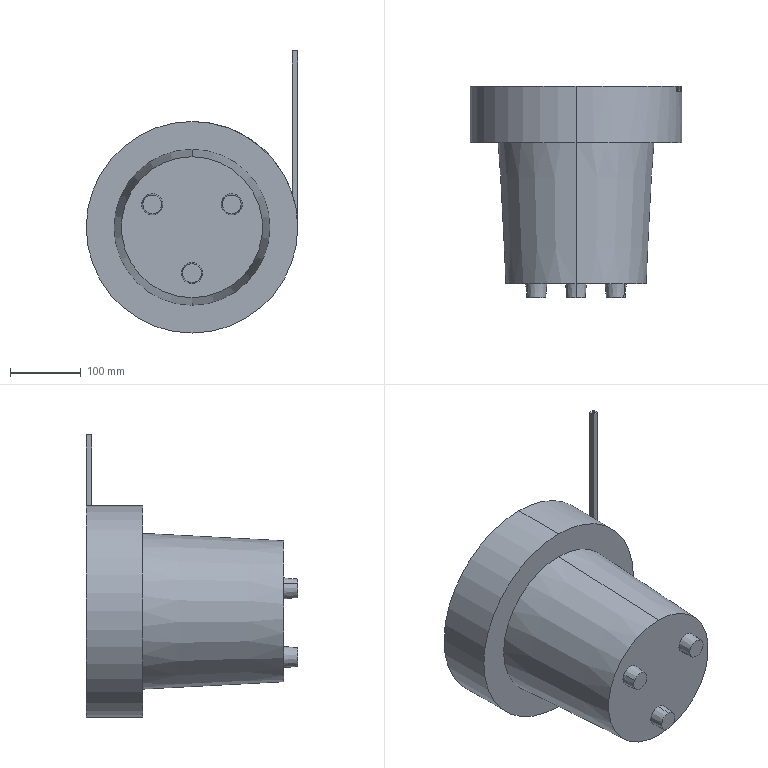Part | NX | features BREP 1 | 1 solid | 40 faces | box 300 x 300 x 400 mm | volume 553756 mm3 | plane 20 | cone 16 | cylinder 4 | commonest cylinder face diameters 296 x2 300 x2
STEP:
#1=CARTESIAN_POINT('',(66.18,-18.,38.209));
#2=VERTEX_POINT('',#1);
#3=CARTESIAN_POINT('',(46.404,-18.,26.791));
#4=VERTEX_POINT('',#3);
#5=CARTESIAN_POINT('',(56.292,-18.,32.5));
#6=DIRECTION('',(0.,-1.,0.));
#7=DIRECTION('',(0.,0.,-1.));
#8=AXIS2_PLACEMENT_3D('',#5,#6,#7);
#9=CIRCLE('',#8,11.418);
#10=EDGE_CURVE('',#2,#4,#9,.T.);
#11=ORIENTED_EDGE('',*,*,#10,.T.);
#12=CARTESIAN_POINT('',(44.888,2.,25.916));
#13=VERTEX_POINT('',#12);
#14=CARTESIAN_POINT('',(45.027,0.1743,25.996));
#15=DIRECTION('',(-0.07548,0.9962,-0.04358));
#16=VECTOR('',#15,1000.);
#17=LINE('',#14,#16);
#18=EDGE_CURVE('',#13,#4,#17,.F.);
#19=ORIENTED_EDGE('',*,*,#18,.F.);
#20=CARTESIAN_POINT('',(67.695,2.,39.084));
#21=VERTEX_POINT('',#20);
#22=CARTESIAN_POINT('',(56.292,2.,32.5));
#23=DIRECTION('',(0.,-1.,0.));
#24=DIRECTION('',(0.,0.,1.));
#25=AXIS2_PLACEMENT_3D('',#22,#23,#24);
#26=CIRCLE('',#25,13.167);
#27=EDGE_CURVE('',#21,#13,#26,.T.);
#28=ORIENTED_EDGE('',*,*,#27,.F.);
#29=CARTESIAN_POINT('',(67.557,0.1743,39.004));
#30=DIRECTION('',(0.07548,0.9962,0.04358));
#31=VECTOR('',#30,1000.);
#32=LINE('',#29,#31);
#33=EDGE_CURVE('',#21,#2,#32,.F.);
#34=ORIENTED_EDGE('',*,*,#33,.T.);
#35=EDGE_LOOP('',(#11,#19,#28,#34));
#36=FACE_BOUND('',#35,.T.);
#37=CARTESIAN_POINT('',(56.292,0.1743,32.5));
#38=DIRECTION('',(0.,1.,0.));
#39=DIRECTION('',(0.866,0.,0.5));
#40=AXIS2_PLACEMENT_3D('',#37,#38,#39);
#41=CONICAL_SURFACE('',#40,13.008,0.08727);
#42=ADVANCED_FACE('',(#36),#41,.F.);
#43=CARTESIAN_POINT('',(-66.18,-18.,38.209));
#44=VERTEX_POINT('',#43);
#45=CARTESIAN_POINT('',(-46.404,-18.,26.791));
#46=VERTEX_POINT('',#45);
#47=CARTESIAN_POINT('',(-56.292,-18.,32.5));
#48=DIRECTION('',(0.,-1.,0.));
#49=DIRECTION('',(0.,0.,-1.));
#50=AXIS2_PLACEMENT_3D('',#47,#48,#49);
#51=CIRCLE('',#50,11.418);
#52=EDGE_CURVE('',#44,#46,#51,.T.);
#53=ORIENTED_EDGE('',*,*,#52,.T.);
#54=CARTESIAN_POINT('',(-44.888,2.,25.916));
#55=VERTEX_POINT('',#54);
#56=CARTESIAN_POINT('',(-45.027,0.1743,25.996));
#57=DIRECTION('',(0.07548,0.9962,-0.04358));
#58=VECTOR('',#57,1000.);
#59=LINE('',#56,#58);
#60=EDGE_CURVE('',#46,#55,#59,.T.);
#61=ORIENTED_EDGE('',*,*,#60,.T.);
#62=CARTESIAN_POINT('',(-67.695,2.,39.084));
#63=VERTEX_POINT('',#62);
#64=CARTESIAN_POINT('',(-56.292,2.,32.5));
#65=DIRECTION('',(0.,-1.,0.));
#66=DIRECTION('',(0.,0.,1.));
#67=AXIS2_PLACEMENT_3D('',#64,#65,#66);
#68=CIRCLE('',#67,13.167);
#69=EDGE_CURVE('',#63,#55,#68,.T.);
#70=ORIENTED_EDGE('',*,*,#69,.F.);
#71=CARTESIAN_POINT('',(-67.557,0.1743,39.004));
#72=DIRECTION('',(-0.07548,0.9962,0.04358));
#73=VECTOR('',#72,1000.);
#74=LINE('',#71,#73);
#75=EDGE_CURVE('',#44,#63,#74,.T.);
#76=ORIENTED_EDGE('',*,*,#75,.F.);
#77=EDGE_LOOP('',(#53,#61,#70,#76));
#78=FACE_BOUND('',#77,.T.);
#79=CARTESIAN_POINT('',(-56.292,0.1743,32.5));
#80=DIRECTION('',(0.,1.,0.));
#81=DIRECTION('',(-0.866,0.,0.5));
#82=AXIS2_PLACEMENT_3D('',#79,#80,#81);
#83=CONICAL_SURFACE('',#82,13.008,0.08727);
#84=ADVANCED_FACE('',(#78),#83,.F.);
#85=CARTESIAN_POINT('',(0.,-18.,-76.418));
#86=VERTEX_POINT('',#85);
#87=CARTESIAN_POINT('',(0.,-18.,-53.582));
#88=VERTEX_POINT('',#87);
#89=CARTESIAN_POINT('',(0.,-18.,-65.));
#90=DIRECTION('',(0.,-1.,0.));
#91=DIRECTION('',(0.,0.,-1.));
#92=AXIS2_PLACEMENT_3D('',#89,#90,#91);
#93=CIRCLE('',#92,11.418);
#94=EDGE_CURVE('',#86,#88,#93,.T.);
#95=ORIENTED_EDGE('',*,*,#94,.T.);
#96=CARTESIAN_POINT('',(0.,2.,-51.833));
#97=VERTEX_POINT('',#96);
#98=CARTESIAN_POINT('',(0.,0.1743,-51.992));
#99=DIRECTION('',(0.,0.9962,0.08716));
#100=VECTOR('',#99,1000.);
#101=LINE('',#98,#100);
#102=EDGE_CURVE('',#88,#97,#101,.T.);
#103=ORIENTED_EDGE('',*,*,#102,.T.);
#104=CARTESIAN_POINT('',(0.,2.,-78.167));
#105=VERTEX_POINT('',#104);
#106=CARTESIAN_POINT('',(0.,2.,-65.));
#107=DIRECTION('',(0.,-1.,0.));
#108=DIRECTION('',(0.,0.,1.));
#109=AXIS2_PLACEMENT_3D('',#106,#107,#108);
#110=CIRCLE('',#109,13.167);
#111=EDGE_CURVE('',#105,#97,#110,.T.);
#112=ORIENTED_EDGE('',*,*,#111,.F.);
#113=CARTESIAN_POINT('',(0.,0.1743,-78.008));
#114=DIRECTION('',(0.,0.9962,-0.08716));
#115=VECTOR('',#114,1000.);
#116=LINE('',#113,#115);
#117=EDGE_CURVE('',#86,#105,#116,.T.);
#118=ORIENTED_EDGE('',*,*,#117,.F.);
#119=EDGE_LOOP('',(#95,#103,#112,#118));
#120=FACE_BOUND('',#119,.T.);
#121=CARTESIAN_POINT('',(0.,0.1743,-65.));
#122=DIRECTION('',(0.,1.,0.));
#123=DIRECTION('',(0.,0.,-1.));
#124=AXIS2_PLACEMENT_3D('',#121,#122,#123);
#125=CONICAL_SURFACE('',#124,13.008,0.08727);
#126=ADVANCED_FACE('',(#120),#125,.F.);
#127=CARTESIAN_POINT('',(0.,2.,-98.102));
#128=VERTEX_POINT('',#127);
#129=CARTESIAN_POINT('',(0.,2.,98.102));
#130=VERTEX_POINT('',#129);
#131=CARTESIAN_POINT('',(0.,2.,0.));
#132=DIRECTION('',(0.,1.,0.));
#133=DIRECTION('',(0.,0.,1.));
#134=AXIS2_PLACEMENT_3D('',#131,#132,#133);
#135=CIRCLE('',#134,98.102);
#136=EDGE_CURVE('',#128,#130,#135,.T.);
#137=ORIENTED_EDGE('',*,*,#136,.F.);
#138=CARTESIAN_POINT('',(0.,202.,-108.584));
#139=VERTEX_POINT('',#138);
#140=CARTESIAN_POINT('',(0.,0.1047,-98.003));
#141=DIRECTION('',(0.,0.9986,-0.05234));
#142=VECTOR('',#141,1000.);
#143=LINE('',#140,#142);
#144=EDGE_CURVE('',#139,#128,#143,.F.);
#145=ORIENTED_EDGE('',*,*,#144,.F.);
#146=CARTESIAN_POINT('',(0.,202.,108.584));
#147=VERTEX_POINT('',#146);
#148=CARTESIAN_POINT('',(0.,202.,0.));
#149=DIRECTION('',(0.,1.,0.));
#150=DIRECTION('',(0.,0.,1.));
#151=AXIS2_PLACEMENT_3D('',#148,#149,#150);
#152=CIRCLE('',#151,108.584);
#153=EDGE_CURVE('',#139,#147,#152,.T.);
#154=ORIENTED_EDGE('',*,*,#153,.T.);
#155=CARTESIAN_POINT('',(0.,0.1047,98.003));
#156=DIRECTION('',(0.,0.9986,0.05234));
#157=VECTOR('',#156,1000.);
#158=LINE('',#155,#157);
#159=EDGE_CURVE('',#147,#130,#158,.F.);
#160=ORIENTED_EDGE('',*,*,#159,.T.);
#161=EDGE_LOOP('',(#137,#145,#154,#160));
#162=FACE_BOUND('',#161,.T.);
#163=CARTESIAN_POINT('',(0.,0.1047,0.));
#164=DIRECTION('',(0.,1.,0.));
#165=DIRECTION('',(0.,0.,1.));
#166=AXIS2_PLACEMENT_3D('',#163,#164,#165);
#167=CONICAL_SURFACE('',#166,98.003,0.05236);
#168=ADVANCED_FACE('',(#162),#167,.F.);
#169=CARTESIAN_POINT('',(0.,280.,-148.));
#170=VERTEX_POINT('',#169);
#171=CARTESIAN_POINT('',(0.,280.,148.));
#172=VERTEX_POINT('',#171);
#173=CARTESIAN_POINT('',(0.,280.,0.));
#174=DIRECTION('',(0.,1.,0.));
#175=DIRECTION('',(0.,0.,1.));
#176=AXIS2_PLACEMENT_3D('',#173,#174,#175);
#177=CIRCLE('',#176,148.);
#178=EDGE_CURVE('',#170,#172,#177,.T.);
#179=ORIENTED_EDGE('',*,*,#178,.T.);
#180=CARTESIAN_POINT('',(0.,202.,148.));
#181=VERTEX_POINT('',#180);
#182=CARTESIAN_POINT('',(0.,280.,148.));
#183=DIRECTION('',(0.,-1.,0.));
#184=VECTOR('',#183,1000.);
#185=LINE('',#182,#184);
#186=EDGE_CURVE('',#172,#181,#185,.T.);
#187=ORIENTED_EDGE('',*,*,#186,.T.);
#188=CARTESIAN_POINT('',(0.,202.,-148.));
#189=VERTEX_POINT('',#188);
#190=CARTESIAN_POINT('',(0.,202.,0.));
#191=DIRECTION('',(0.,1.,0.));
#192=DIRECTION('',(0.,0.,1.));
#193=AXIS2_PLACEMENT_3D('',#190,#191,#192);
#194=CIRCLE('',#193,148.);
#195=EDGE_CURVE('',#189,#181,#194,.T.);
#196=ORIENTED_EDGE('',*,*,#195,.F.);
#197=CARTESIAN_POINT('',(0.,280.,-148.));
#198=DIRECTION('',(0.,-1.,0.));
#199=VECTOR('',#198,1000.);
#200=LINE('',#197,#199);
#201=EDGE_CURVE('',#170,#189,#200,.T.);
#202=ORIENTED_EDGE('',*,*,#201,.F.);
#203=EDGE_LOOP('',(#179,#187,#196,#202));
#204=FACE_BOUND('',#203,.T.);
#205=CARTESIAN_POINT('',(0.,280.,0.));
#206=DIRECTION('',(0.,-1.,0.));
#207=DIRECTION('',(0.,0.,-1.));
#208=AXIS2_PLACEMENT_3D('',#205,#206,#207);
#209=CYLINDRICAL_SURFACE('',#208,148.);
#210=ADVANCED_FACE('',(#204),#209,.F.);
#211=CARTESIAN_POINT('',(44.817,-20.,25.875));
#212=VERTEX_POINT('',#211);
#213=CARTESIAN_POINT('',(67.767,-20.,39.125));
#214=VERTEX_POINT('',#213);
#215=CARTESIAN_POINT('',(56.292,-20.,32.5));
#216=DIRECTION('',(0.,-1.,0.));
#217=DIRECTION('',(0.,0.,-1.));
#218=AXIS2_PLACEMENT_3D('',#215,#216,#217);
#219=CIRCLE('',#218,13.25);
#220=EDGE_CURVE('',#212,#214,#219,.T.);
#221=ORIENTED_EDGE('',*,*,#220,.F.);
#222=CARTESIAN_POINT('',(43.301,0.,25.));
#223=VERTEX_POINT('',#222);
#224=CARTESIAN_POINT('',(43.301,0.,25.));
#225=DIRECTION('',(-0.07548,0.9962,-0.04358));
#226=VECTOR('',#225,1000.);
#227=LINE('',#224,#226);
#228=EDGE_CURVE('',#223,#212,#227,.F.);
#229=ORIENTED_EDGE('',*,*,#228,.F.);
#230=CARTESIAN_POINT('',(69.282,0.,40.));
#231=VERTEX_POINT('',#230);
#232=CARTESIAN_POINT('',(56.292,0.,32.5));
#233=DIRECTION('',(0.,-1.,0.));
#234=DIRECTION('',(0.,0.,1.));
#235=AXIS2_PLACEMENT_3D('',#232,#233,#234);
#236=CIRCLE('',#235,15.);
#237=EDGE_CURVE('',#223,#231,#236,.T.);
#238=ORIENTED_EDGE('',*,*,#237,.T.);
#239=CARTESIAN_POINT('',(69.282,0.,40.));
#240=DIRECTION('',(0.07548,0.9962,0.04358));
#241=VECTOR('',#240,1000.);
#242=LINE('',#239,#241);
#243=EDGE_CURVE('',#231,#214,#242,.F.);
#244=ORIENTED_EDGE('',*,*,#243,.T.);
#245=EDGE_LOOP('',(#221,#229,#238,#244));
#246=FACE_BOUND('',#245,.T.);
#247=CARTESIAN_POINT('',(56.292,0.,32.5));
#248=DIRECTION('',(0.,1.,0.));
#249=DIRECTION('',(0.866,0.,0.5));
#250=AXIS2_PLACEMENT_3D('',#247,#248,#249);
#251=CONICAL_SURFACE('',#250,15.,0.08727);
#252=ADVANCED_FACE('',(#246),#251,.T.);
#253=CARTESIAN_POINT('',(-44.817,-20.,25.875));
#254=VERTEX_POINT('',#253);
#255=CARTESIAN_POINT('',(-67.767,-20.,39.125));
#256=VERTEX_POINT('',#255);
#257=CARTESIAN_POINT('',(-56.292,-20.,32.5));
#258=DIRECTION('',(0.,-1.,0.));
#259=DIRECTION('',(0.,0.,-1.));
#260=AXIS2_PLACEMENT_3D('',#257,#258,#259);
#261=CIRCLE('',#260,13.25);
#262=EDGE_CURVE('',#254,#256,#261,.T.);
#263=ORIENTED_EDGE('',*,*,#262,.F.);
#264=CARTESIAN_POINT('',(-43.301,0.,25.));
#265=VERTEX_POINT('',#264);
#266=CARTESIAN_POINT('',(-43.301,0.,25.));
#267=DIRECTION('',(0.07548,0.9962,-0.04358));
#268=VECTOR('',#267,1000.);
#269=LINE('',#266,#268);
#270=EDGE_CURVE('',#254,#265,#269,.T.);
#271=ORIENTED_EDGE('',*,*,#270,.T.);
#272=CARTESIAN_POINT('',(-69.282,0.,40.));
#273=VERTEX_POINT('',#272);
#274=CARTESIAN_POINT('',(-56.292,0.,32.5));
#275=DIRECTION('',(0.,-1.,0.));
#276=DIRECTION('',(0.,0.,1.));
#277=AXIS2_PLACEMENT_3D('',#274,#275,#276);
#278=CIRCLE('',#277,15.);
#279=EDGE_CURVE('',#265,#273,#278,.T.);
#280=ORIENTED_EDGE('',*,*,#279,.T.);
#281=CARTESIAN_POINT('',(-69.282,0.,40.));
#282=DIRECTION('',(-0.07548,0.9962,0.04358));
#283=VECTOR('',#282,1000.);
#284=LINE('',#281,#283);
#285=EDGE_CURVE('',#256,#273,#284,.T.);
#286=ORIENTED_EDGE('',*,*,#285,.F.);
#287=EDGE_LOOP('',(#263,#271,#280,#286));
#288=FACE_BOUND('',#287,.T.);
#289=CARTESIAN_POINT('',(-56.292,0.,32.5));
#290=DIRECTION('',(0.,1.,0.));
#291=DIRECTION('',(-0.866,0.,0.5));
#292=AXIS2_PLACEMENT_3D('',#289,#290,#291);
#293=CONICAL_SURFACE('',#292,15.,0.08727);
#294=ADVANCED_FACE('',(#288),#293,.T.);
#295=CARTESIAN_POINT('',(0.,-20.,-51.75));
#296=VERTEX_POINT('',#295);
#297=CARTESIAN_POINT('',(0.,-20.,-78.25));
#298=VERTEX_POINT('',#297);
#299=CARTESIAN_POINT('',(0.,-20.,-65.));
#300=DIRECTION('',(0.,-1.,0.));
#301=DIRECTION('',(0.,0.,-1.));
#302=AXIS2_PLACEMENT_3D('',#299,#300,#301);
#303=CIRCLE('',#302,13.25);
#304=EDGE_CURVE('',#296,#298,#303,.T.);
#305=ORIENTED_EDGE('',*,*,#304,.F.);
#306=CARTESIAN_POINT('',(0.,0.,-50.));
#307=VERTEX_POINT('',#306);
#308=CARTESIAN_POINT('',(0.,0.,-50.));
#309=DIRECTION('',(0.,0.9962,0.08716));
#310=VECTOR('',#309,1000.);
#311=LINE('',#308,#310);
#312=EDGE_CURVE('',#296,#307,#311,.T.);
#313=ORIENTED_EDGE('',*,*,#312,.T.);
#314=CARTESIAN_POINT('',(0.,0.,-80.));
#315=VERTEX_POINT('',#314);
#316=CARTESIAN_POINT('',(0.,0.,-65.));
#317=DIRECTION('',(0.,-1.,0.));
#318=DIRECTION('',(0.,0.,1.));
#319=AXIS2_PLACEMENT_3D('',#316,#317,#318);
#320=CIRCLE('',#319,15.);
#321=EDGE_CURVE('',#307,#315,#320,.T.);
#322=ORIENTED_EDGE('',*,*,#321,.T.);
#323=CARTESIAN_POINT('',(0.,0.,-80.));
#324=DIRECTION('',(0.,0.9962,-0.08716));
#325=VECTOR('',#324,1000.);
#326=LINE('',#323,#325);
#327=EDGE_CURVE('',#298,#315,#326,.T.);
#328=ORIENTED_EDGE('',*,*,#327,.F.);
#329=EDGE_LOOP('',(#305,#313,#322,#328));
#330=FACE_BOUND('',#329,.T.);
#331=CARTESIAN_POINT('',(0.,0.,-65.));
#332=DIRECTION('',(0.,1.,0.));
#333=DIRECTION('',(0.,0.,-1.));
#334=AXIS2_PLACEMENT_3D('',#331,#332,#333);
#335=CONICAL_SURFACE('',#334,15.,0.08727);
#336=ADVANCED_FACE('',(#330),#335,.T.);
#337=CARTESIAN_POINT('',(0.,0.,100.));
#338=VERTEX_POINT('',#337);
#339=CARTESIAN_POINT('',(0.,0.,-100.));
#340=VERTEX_POINT('',#339);
#341=CARTESIAN_POINT('',(0.,0.,0.));
#342=DIRECTION('',(0.,1.,0.));
#343=DIRECTION('',(0.,0.,1.));
#344=AXIS2_PLACEMENT_3D('',#341,#342,#343);
#345=CIRCLE('',#344,100.);
#346=EDGE_CURVE('',#338,#340,#345,.T.);
#347=ORIENTED_EDGE('',*,*,#346,.T.);
#348=CARTESIAN_POINT('',(0.,200.,-110.482));
#349=VERTEX_POINT('',#348);
#350=CARTESIAN_POINT('',(0.,0.,-100.));
#351=DIRECTION('',(0.,0.9986,-0.05234));
#352=VECTOR('',#351,1000.);
#353=LINE('',#350,#352);
#354=EDGE_CURVE('',#349,#340,#353,.F.);
#355=ORIENTED_EDGE('',*,*,#354,.F.);
#356=CARTESIAN_POINT('',(0.,200.,110.482));
#357=VERTEX_POINT('',#356);
#358=CARTESIAN_POINT('',(0.,200.,0.));
#359=DIRECTION('',(0.,1.,0.));
#360=DIRECTION('',(0.,0.,1.));
#361=AXIS2_PLACEMENT_3D('',#358,#359,#360);
#362=CIRCLE('',#361,110.482);
#363=EDGE_CURVE('',#357,#349,#362,.T.);
#364=ORIENTED_EDGE('',*,*,#363,.F.);
#365=CARTESIAN_POINT('',(0.,0.,100.));
#366=DIRECTION('',(0.,0.9986,0.05234));
#367=VECTOR('',#366,1000.);
#368=LINE('',#365,#367);
#369=EDGE_CURVE('',#357,#338,#368,.F.);
#370=ORIENTED_EDGE('',*,*,#369,.T.);
#371=EDGE_LOOP('',(#347,#355,#364,#370));
#372=FACE_BOUND('',#371,.T.);
#373=CARTESIAN_POINT('',(0.,0.,0.));
#374=DIRECTION('',(0.,1.,0.));
#375=DIRECTION('',(0.,0.,1.));
#376=AXIS2_PLACEMENT_3D('',#373,#374,#375);
#377=CONICAL_SURFACE('',#376,100.,0.05236);
#378=ADVANCED_FACE('',(#372),#377,.T.);
#379=CARTESIAN_POINT('',(0.,280.,150.));
#380=VERTEX_POINT('',#379);
#381=CARTESIAN_POINT('',(142.,280.,48.332));
#382=VERTEX_POINT('',#381);
#383=CARTESIAN_POINT('',(0.,280.,0.));
#384=DIRECTION('',(0.,1.,0.));
#385=DIRECTION('',(0.,0.,1.));
#386=AXIS2_PLACEMENT_3D('',#383,#384,#385);
#387=CIRCLE('',#386,150.);
#388=EDGE_CURVE('',#380,#382,#387,.T.);
#389=ORIENTED_EDGE('',*,*,#388,.F.);
#390=CARTESIAN_POINT('',(0.,200.,150.));
#391=VERTEX_POINT('',#390);
#392=CARTESIAN_POINT('',(0.,280.,150.));
#393=DIRECTION('',(0.,-1.,0.));
#394=VECTOR('',#393,1000.);
#395=LINE('',#392,#394);
#396=EDGE_CURVE('',#380,#391,#395,.T.);
#397=ORIENTED_EDGE('',*,*,#396,.T.);
#398=CARTESIAN_POINT('',(0.,200.,-150.));
#399=VERTEX_POINT('',#398);
#400=CARTESIAN_POINT('',(0.,200.,0.));
#401=DIRECTION('',(0.,1.,0.));
#402=DIRECTION('',(0.,0.,1.));
#403=AXIS2_PLACEMENT_3D('',#400,#401,#402);
#404=CIRCLE('',#403,150.);
#405=EDGE_CURVE('',#391,#399,#404,.T.);
#406=ORIENTED_EDGE('',*,*,#405,.T.);
#407=CARTESIAN_POINT('',(0.,280.,-150.));
#408=VERTEX_POINT('',#407);
#409=CARTESIAN_POINT('',(0.,280.,-150.));
#410=DIRECTION('',(0.,-1.,0.));
#411=VECTOR('',#410,1000.);
#412=LINE('',#409,#411);
#413=EDGE_CURVE('',#408,#399,#412,.T.);
#414=ORIENTED_EDGE('',*,*,#413,.F.);
#415=CARTESIAN_POINT('',(150.,280.,0.));
#416=VERTEX_POINT('',#415);
#417=CARTESIAN_POINT('',(0.,280.,0.));
#418=DIRECTION('',(0.,1.,0.));
#419=DIRECTION('',(0.,0.,1.));
#420=AXIS2_PLACEMENT_3D('',#417,#418,#419);
#421=CIRCLE('',#420,150.);
#422=EDGE_CURVE('',#416,#408,#421,.T.);
#423=ORIENTED_EDGE('',*,*,#422,.F.);
#424=CARTESIAN_POINT('',(150.,272.,0.));
#425=VERTEX_POINT('',#424);
#426=CARTESIAN_POINT('',(150.,280.,0.));
#427=DIRECTION('',(0.,1.,0.));
#428=VECTOR('',#427,1000.);
#429=LINE('',#426,#428);
#430=EDGE_CURVE('',#425,#416,#429,.T.);
#431=ORIENTED_EDGE('',*,*,#430,.F.);
#432=CARTESIAN_POINT('',(142.,272.,48.332));
#433=VERTEX_POINT('',#432);
#434=CARTESIAN_POINT('',(0.,272.,0.));
#435=DIRECTION('',(0.,1.,0.));
#436=DIRECTION('',(0.,0.,1.));
#437=AXIS2_PLACEMENT_3D('',#434,#435,#436);
#438=CIRCLE('',#437,150.);
#439=EDGE_CURVE('',#433,#425,#438,.T.);
#440=ORIENTED_EDGE('',*,*,#439,.F.);
#441=CARTESIAN_POINT('',(142.,280.,48.332));
#442=DIRECTION('',(0.,-1.,0.));
#443=VECTOR('',#442,1000.);
#444=LINE('',#441,#443);
#445=EDGE_CURVE('',#382,#433,#444,.T.);
#446=ORIENTED_EDGE('',*,*,#445,.F.);
#447=EDGE_LOOP('',(#389,#397,#406,#414,#423,#431,#440,#446));
#448=FACE_BOUND('',#447,.T.);
#449=CARTESIAN_POINT('',(0.,280.,0.));
#450=DIRECTION('',(0.,-1.,0.));
#451=DIRECTION('',(0.,0.,-1.));
#452=AXIS2_PLACEMENT_3D('',#449,#450,#451);
#453=CYLINDRICAL_SURFACE('',#452,150.);
#454=ADVANCED_FACE('',(#448),#453,.T.);
#455=ORIENTED_EDGE('',*,*,#396,.F.);
#456=CARTESIAN_POINT('',(0.,280.,0.));
#457=DIRECTION('',(0.,1.,0.));
#458=DIRECTION('',(0.,0.,1.));
#459=AXIS2_PLACEMENT_3D('',#456,#457,#458);
#460=CIRCLE('',#459,150.);
#461=EDGE_CURVE('',#408,#380,#460,.T.);
#462=ORIENTED_EDGE('',*,*,#461,.F.);
#463=ORIENTED_EDGE('',*,*,#413,.T.);
#464=CARTESIAN_POINT('',(0.,200.,0.));
#465=DIRECTION('',(0.,1.,0.));
#466=DIRECTION('',(0.,0.,1.));
#467=AXIS2_PLACEMENT_3D('',#464,#465,#466);
#468=CIRCLE('',#467,150.);
#469=EDGE_CURVE('',#399,#391,#468,.T.);
#470=ORIENTED_EDGE('',*,*,#469,.T.);
#471=EDGE_LOOP('',(#455,#462,#463,#470));
#472=FACE_BOUND('',#471,.T.);
#473=CARTESIAN_POINT('',(0.,280.,0.));
#474=DIRECTION('',(0.,-1.,0.));
#475=DIRECTION('',(0.,0.,-1.));
#476=AXIS2_PLACEMENT_3D('',#473,#474,#475);
#477=CYLINDRICAL_SURFACE('',#476,150.);
#478=ADVANCED_FACE('',(#472),#477,.T.);
#479=ORIENTED_EDGE('',*,*,#346,.F.);
#480=CARTESIAN_POINT('',(0.,0.,0.));
#481=DIRECTION('',(0.,1.,0.));
#482=DIRECTION('',(0.,0.,1.));
#483=AXIS2_PLACEMENT_3D('',#480,#481,#482);
#484=CIRCLE('',#483,100.);
#485=EDGE_CURVE('',#340,#338,#484,.T.);
#486=ORIENTED_EDGE('',*,*,#485,.F.);
#487=EDGE_LOOP('',(#479,#486));
#488=FACE_BOUND('',#487,.T.);
#489=CARTESIAN_POINT('',(-56.292,0.,32.5));
#490=DIRECTION('',(0.,-1.,0.));
#491=DIRECTION('',(0.,0.,1.));
#492=AXIS2_PLACEMENT_3D('',#489,#490,#491);
#493=CIRCLE('',#492,15.);
#494=EDGE_CURVE('',#273,#265,#493,.T.);
#495=ORIENTED_EDGE('',*,*,#494,.F.);
#496=ORIENTED_EDGE('',*,*,#279,.F.);
#497=EDGE_LOOP('',(#495,#496));
#498=FACE_BOUND('',#497,.T.);
#499=CARTESIAN_POINT('',(0.,0.,-65.));
#500=DIRECTION('',(0.,-1.,0.));
#501=DIRECTION('',(0.,0.,1.));
#502=AXIS2_PLACEMENT_3D('',#499,#500,#501);
#503=CIRCLE('',#502,15.);
#504=EDGE_CURVE('',#315,#307,#503,.T.);
#505=ORIENTED_EDGE('',*,*,#504,.F.);
#506=ORIENTED_EDGE('',*,*,#321,.F.);
#507=EDGE_LOOP('',(#505,#506));
#508=FACE_BOUND('',#507,.T.);
#509=CARTESIAN_POINT('',(56.292,0.,32.5));
#510=DIRECTION('',(0.,-1.,0.));
#511=DIRECTION('',(0.,0.,1.));
#512=AXIS2_PLACEMENT_3D('',#509,#510,#511);
#513=CIRCLE('',#512,15.);
#514=EDGE_CURVE('',#231,#223,#513,.T.);
#515=ORIENTED_EDGE('',*,*,#514,.F.);
#516=ORIENTED_EDGE('',*,*,#237,.F.);
#517=EDGE_LOOP('',(#515,#516));
#518=FACE_BOUND('',#517,.T.);
#519=CARTESIAN_POINT('',(0.,0.,0.));
#520=DIRECTION('',(0.,1.,0.));
#521=DIRECTION('',(1.,0.,0.));
#522=AXIS2_PLACEMENT_3D('',#519,#520,#521);
#523=PLANE('',#522);
#524=ADVANCED_FACE('',(#488,#498,#508,#518),#523,.F.);
#525=ORIENTED_EDGE('',*,*,#354,.T.);
#526=ORIENTED_EDGE('',*,*,#485,.T.);
#527=ORIENTED_EDGE('',*,*,#369,.F.);
#528=CARTESIAN_POINT('',(0.,200.,0.));
#529=DIRECTION('',(0.,1.,0.));
#530=DIRECTION('',(0.,0.,1.));
#531=AXIS2_PLACEMENT_3D('',#528,#529,#530);
#532=CIRCLE('',#531,110.482);
#533=EDGE_CURVE('',#349,#357,#532,.T.);
#534=ORIENTED_EDGE('',*,*,#533,.F.);
#535=EDGE_LOOP('',(#525,#526,#527,#534));
#536=FACE_BOUND('',#535,.T.);
#537=CARTESIAN_POINT('',(0.,0.,0.));
#538=DIRECTION('',(0.,1.,0.));
#539=DIRECTION('',(0.,0.,1.));
#540=AXIS2_PLACEMENT_3D('',#537,#538,#539);
#541=CONICAL_SURFACE('',#540,100.,0.05236);
#542=ADVANCED_FACE('',(#536),#541,.T.);
#543=ORIENTED_EDGE('',*,*,#469,.F.);
#544=ORIENTED_EDGE('',*,*,#405,.F.);
#545=EDGE_LOOP('',(#543,#544));
#546=FACE_BOUND('',#545,.T.);
#547=ORIENTED_EDGE('',*,*,#363,.T.);
#548=ORIENTED_EDGE('',*,*,#533,.T.);
#549=EDGE_LOOP('',(#547,#548));
#550=FACE_BOUND('',#549,.T.);
#551=CARTESIAN_POINT('',(0.,200.,0.));
#552=DIRECTION('',(0.,1.,0.));
#553=DIRECTION('',(1.,0.,0.));
#554=AXIS2_PLACEMENT_3D('',#551,#552,#553);
#555=PLANE('',#554);
#556=ADVANCED_FACE('',(#546,#550),#555,.F.);
#557=CARTESIAN_POINT('',(144.,280.,250.));
#558=VERTEX_POINT('',#557);
#559=CARTESIAN_POINT('',(142.,280.,250.));
#560=VERTEX_POINT('',#559);
#561=CARTESIAN_POINT('',(142.,280.,250.));
#562=DIRECTION('',(-1.,0.,0.));
#563=VECTOR('',#562,1000.);
#564=LINE('',#561,#563);
#565=EDGE_CURVE('',#558,#560,#564,.T.);
#566=ORIENTED_EDGE('',*,*,#565,.F.);
#567=CARTESIAN_POINT('',(144.,280.,34.176));
#568=VERTEX_POINT('',#567);
#569=CARTESIAN_POINT('',(144.,280.,0.));
#570=DIRECTION('',(0.,0.,-1.));
#571=VECTOR('',#570,1000.);
#572=LINE('',#569,#571);
#573=EDGE_CURVE('',#558,#568,#572,.T.);
#574=ORIENTED_EDGE('',*,*,#573,.T.);
#575=CARTESIAN_POINT('',(0.,280.,0.));
#576=DIRECTION('',(0.,1.,0.));
#577=DIRECTION('',(0.,0.,1.));
#578=AXIS2_PLACEMENT_3D('',#575,#576,#577);
#579=CIRCLE('',#578,148.);
#580=EDGE_CURVE('',#172,#568,#579,.T.);
#581=ORIENTED_EDGE('',*,*,#580,.F.);
#582=ORIENTED_EDGE('',*,*,#178,.F.);
#583=CARTESIAN_POINT('',(148.,280.,0.));
#584=VERTEX_POINT('',#583);
#585=CARTESIAN_POINT('',(0.,280.,0.));
#586=DIRECTION('',(0.,1.,0.));
#587=DIRECTION('',(0.,0.,1.));
#588=AXIS2_PLACEMENT_3D('',#585,#586,#587);
#589=CIRCLE('',#588,148.);
#590=EDGE_CURVE('',#584,#170,#589,.T.);
#591=ORIENTED_EDGE('',*,*,#590,.F.);
#592=CARTESIAN_POINT('',(148.,280.,248.));
#593=VERTEX_POINT('',#592);
#594=CARTESIAN_POINT('',(148.,280.,250.));
#595=DIRECTION('',(0.,0.,-1.));
#596=VECTOR('',#595,1000.);
#597=LINE('',#594,#596);
#598=EDGE_CURVE('',#593,#584,#597,.T.);
#599=ORIENTED_EDGE('',*,*,#598,.F.);
#600=CARTESIAN_POINT('',(147.993,280.,248.));
#601=VERTEX_POINT('',#600);
#602=CARTESIAN_POINT('',(0.,280.,248.));
#603=DIRECTION('',(-1.,0.,0.));
#604=VECTOR('',#603,1000.);
#605=LINE('',#602,#604);
#606=EDGE_CURVE('',#593,#601,#605,.T.);
#607=ORIENTED_EDGE('',*,*,#606,.T.);
#608=CARTESIAN_POINT('',(147.993,280.,250.));
#609=VERTEX_POINT('',#608);
#610=CARTESIAN_POINT('',(147.993,280.,248.));
#611=DIRECTION('',(0.,0.,-1.));
#612=VECTOR('',#611,1000.);
#613=LINE('',#610,#612);
#614=EDGE_CURVE('',#609,#601,#613,.T.);
#615=ORIENTED_EDGE('',*,*,#614,.F.);
#616=CARTESIAN_POINT('',(150.,280.,250.));
#617=VERTEX_POINT('',#616);
#618=CARTESIAN_POINT('',(142.,280.,250.));
#619=DIRECTION('',(-1.,0.,0.));
#620=VECTOR('',#619,1000.);
#621=LINE('',#618,#620);
#622=EDGE_CURVE('',#617,#609,#621,.T.);
#623=ORIENTED_EDGE('',*,*,#622,.F.);
#624=CARTESIAN_POINT('',(150.,280.,250.));
#625=DIRECTION('',(0.,0.,-1.));
#626=VECTOR('',#625,1000.);
#627=LINE('',#624,#626);
#628=EDGE_CURVE('',#617,#416,#627,.T.);
#629=ORIENTED_EDGE('',*,*,#628,.T.);
#630=ORIENTED_EDGE('',*,*,#422,.T.);
#631=ORIENTED_EDGE('',*,*,#461,.T.);
#632=ORIENTED_EDGE('',*,*,#388,.T.);
#633=CARTESIAN_POINT('',(142.,280.,250.));
#634=DIRECTION('',(0.,0.,-1.));
#635=VECTOR('',#634,1000.);
#636=LINE('',#633,#635);
#637=EDGE_CURVE('',#560,#382,#636,.T.);
#638=ORIENTED_EDGE('',*,*,#637,.F.);
#639=EDGE_LOOP('',(#566,#574,#581,#582,#591,#599,#607,#615,#623,#629,#630,#631,#632,#638));
#640=FACE_BOUND('',#639,.T.);
#641=CARTESIAN_POINT('',(0.,280.,0.));
#642=DIRECTION('',(0.,1.,0.));
#643=DIRECTION('',(1.,0.,0.));
#644=AXIS2_PLACEMENT_3D('',#641,#642,#643);
#645=PLANE('',#644);
#646=ADVANCED_FACE('',(#640),#645,.T.);
#647=ORIENTED_EDGE('',*,*,#312,.F.);
#648=CARTESIAN_POINT('',(0.,-20.,-65.));
#649=DIRECTION('',(0.,-1.,0.));
#650=DIRECTION('',(0.,0.,-1.));
#651=AXIS2_PLACEMENT_3D('',#648,#649,#650);
#652=CIRCLE('',#651,13.25);
#653=EDGE_CURVE('',#298,#296,#652,.T.);
#654=ORIENTED_EDGE('',*,*,#653,.F.);
#655=ORIENTED_EDGE('',*,*,#327,.T.);
#656=ORIENTED_EDGE('',*,*,#504,.T.);
#657=EDGE_LOOP('',(#647,#654,#655,#656));
#658=FACE_BOUND('',#657,.T.);
#659=CARTESIAN_POINT('',(0.,0.,-65.));
#660=DIRECTION('',(0.,1.,0.));
#661=DIRECTION('',(0.,0.,-1.));
#662=AXIS2_PLACEMENT_3D('',#659,#660,#661);
#663=CONICAL_SURFACE('',#662,15.,0.08727);
#664=ADVANCED_FACE('',(#658),#663,.T.);
#665=ORIENTED_EDGE('',*,*,#653,.T.);
#666=ORIENTED_EDGE('',*,*,#304,.T.);
#667=EDGE_LOOP('',(#665,#666));
#668=FACE_BOUND('',#667,.T.);
#669=CARTESIAN_POINT('',(0.,-20.,-65.));
#670=DIRECTION('',(0.,-1.,0.));
#671=DIRECTION('',(0.,0.,-1.));
#672=AXIS2_PLACEMENT_3D('',#669,#670,#671);
#673=PLANE('',#672);
#674=ADVANCED_FACE('',(#668),#673,.T.);
#675=ORIENTED_EDGE('',*,*,#270,.F.);
#676=CARTESIAN_POINT('',(-56.292,-20.,32.5));
#677=DIRECTION('',(0.,-1.,0.));
#678=DIRECTION('',(0.,0.,-1.));
#679=AXIS2_PLACEMENT_3D('',#676,#677,#678);
#680=CIRCLE('',#679,13.25);
#681=EDGE_CURVE('',#256,#254,#680,.T.);
#682=ORIENTED_EDGE('',*,*,#681,.F.);
#683=ORIENTED_EDGE('',*,*,#285,.T.);
#684=ORIENTED_EDGE('',*,*,#494,.T.);
#685=EDGE_LOOP('',(#675,#682,#683,#684));
#686=FACE_BOUND('',#685,.T.);
#687=CARTESIAN_POINT('',(-56.292,0.,32.5));
#688=DIRECTION('',(0.,1.,0.));
#689=DIRECTION('',(-0.866,0.,0.5));
#690=AXIS2_PLACEMENT_3D('',#687,#688,#689);
#691=CONICAL_SURFACE('',#690,15.,0.08727);
#692=ADVANCED_FACE('',(#686),#691,.T.);
#693=ORIENTED_EDGE('',*,*,#681,.T.);
#694=ORIENTED_EDGE('',*,*,#262,.T.);
#695=EDGE_LOOP('',(#693,#694));
#696=FACE_BOUND('',#695,.T.);
#697=CARTESIAN_POINT('',(-56.292,-20.,32.5));
#698=DIRECTION('',(0.,-1.,0.));
#699=DIRECTION('',(0.,0.,-1.));
#700=AXIS2_PLACEMENT_3D('',#697,#698,#699);
#701=PLANE('',#700);
#702=ADVANCED_FACE('',(#696),#701,.T.);
#703=ORIENTED_EDGE('',*,*,#228,.T.);
#704=CARTESIAN_POINT('',(56.292,-20.,32.5));
#705=DIRECTION('',(0.,-1.,0.));
#706=DIRECTION('',(0.,0.,-1.));
#707=AXIS2_PLACEMENT_3D('',#704,#705,#706);
#708=CIRCLE('',#707,13.25);
#709=EDGE_CURVE('',#214,#212,#708,.T.);
#710=ORIENTED_EDGE('',*,*,#709,.F.);
#711=ORIENTED_EDGE('',*,*,#243,.F.);
#712=ORIENTED_EDGE('',*,*,#514,.T.);
#713=EDGE_LOOP('',(#703,#710,#711,#712));
#714=FACE_BOUND('',#713,.T.);
#715=CARTESIAN_POINT('',(56.292,0.,32.5));
#716=DIRECTION('',(0.,1.,0.));
#717=DIRECTION('',(0.866,0.,0.5));
#718=AXIS2_PLACEMENT_3D('',#715,#716,#717);
#719=CONICAL_SURFACE('',#718,15.,0.08727);
#720=ADVANCED_FACE('',(#714),#719,.T.);
#721=ORIENTED_EDGE('',*,*,#709,.T.);
#722=ORIENTED_EDGE('',*,*,#220,.T.);
#723=EDGE_LOOP('',(#721,#722));
#724=FACE_BOUND('',#723,.T.);
#725=CARTESIAN_POINT('',(56.292,-20.,32.5));
#726=DIRECTION('',(0.,-1.,0.));
#727=DIRECTION('',(0.,0.,-1.));
#728=AXIS2_PLACEMENT_3D('',#725,#726,#727);
#729=PLANE('',#728);
#730=ADVANCED_FACE('',(#724),#729,.T.);
#731=CARTESIAN_POINT('',(142.,272.,250.));
#732=VERTEX_POINT('',#731);
#733=CARTESIAN_POINT('',(142.,272.,250.));
#734=DIRECTION('',(0.,0.,-1.));
#735=VECTOR('',#734,1000.);
#736=LINE('',#733,#735);
#737=EDGE_CURVE('',#732,#433,#736,.T.);
#738=ORIENTED_EDGE('',*,*,#737,.T.);
#739=ORIENTED_EDGE('',*,*,#439,.T.);
#740=CARTESIAN_POINT('',(150.,272.,250.));
#741=VERTEX_POINT('',#740);
#742=CARTESIAN_POINT('',(150.,272.,250.));
#743=DIRECTION('',(0.,0.,-1.));
#744=VECTOR('',#743,1000.);
#745=LINE('',#742,#744);
#746=EDGE_CURVE('',#741,#425,#745,.T.);
#747=ORIENTED_EDGE('',*,*,#746,.F.);
#748=CARTESIAN_POINT('',(142.,272.,250.));
#749=DIRECTION('',(1.,0.,0.));
#750=VECTOR('',#749,1000.);
#751=LINE('',#748,#750);
#752=EDGE_CURVE('',#732,#741,#751,.T.);
#753=ORIENTED_EDGE('',*,*,#752,.F.);
#754=EDGE_LOOP('',(#738,#739,#747,#753));
#755=FACE_BOUND('',#754,.T.);
#756=CARTESIAN_POINT('',(142.,272.,250.));
#757=DIRECTION('',(0.,1.,0.));
#758=DIRECTION('',(1.,0.,0.));
#759=AXIS2_PLACEMENT_3D('',#756,#757,#758);
#760=PLANE('',#759);
#761=ADVANCED_FACE('',(#755),#760,.F.);
#762=ORIENTED_EDGE('',*,*,#637,.T.);
#763=ORIENTED_EDGE('',*,*,#445,.T.);
#764=ORIENTED_EDGE('',*,*,#737,.F.);
#765=CARTESIAN_POINT('',(142.,280.,250.));
#766=DIRECTION('',(0.,-1.,0.));
#767=VECTOR('',#766,1000.);
#768=LINE('',#765,#767);
#769=EDGE_CURVE('',#560,#732,#768,.T.);
#770=ORIENTED_EDGE('',*,*,#769,.F.);
#771=EDGE_LOOP('',(#762,#763,#764,#770));
#772=FACE_BOUND('',#771,.T.);
#773=CARTESIAN_POINT('',(142.,280.,250.));
#774=DIRECTION('',(1.,0.,0.));
#775=DIRECTION('',(0.,1.,0.));
#776=AXIS2_PLACEMENT_3D('',#773,#774,#775);
#777=PLANE('',#776);
#778=ADVANCED_FACE('',(#772),#777,.F.);
#779=ORIENTED_EDGE('',*,*,#430,.T.);
#780=ORIENTED_EDGE('',*,*,#628,.F.);
#781=CARTESIAN_POINT('',(150.,280.,250.));
#782=DIRECTION('',(0.,1.,0.));
#783=VECTOR('',#782,1000.);
#784=LINE('',#781,#783);
#785=EDGE_CURVE('',#741,#617,#784,.T.);
#786=ORIENTED_EDGE('',*,*,#785,.F.);
#787=ORIENTED_EDGE('',*,*,#746,.T.);
#788=EDGE_LOOP('',(#779,#780,#786,#787));
#789=FACE_BOUND('',#788,.T.);
#790=CARTESIAN_POINT('',(150.,280.,250.));
#791=DIRECTION('',(-1.,0.,0.));
#792=DIRECTION('',(0.,0.,1.));
#793=AXIS2_PLACEMENT_3D('',#790,#791,#792);
#794=PLANE('',#793);
#795=ADVANCED_FACE('',(#789),#794,.F.);
#796=CARTESIAN_POINT('',(144.,274.,250.));
#797=VERTEX_POINT('',#796);
#798=CARTESIAN_POINT('',(144.,0.,250.));
#799=DIRECTION('',(0.,-1.,0.));
#800=VECTOR('',#799,1000.);
#801=LINE('',#798,#800);
#802=EDGE_CURVE('',#558,#797,#801,.T.);
#803=ORIENTED_EDGE('',*,*,#802,.F.);
#804=ORIENTED_EDGE('',*,*,#565,.T.);
#805=ORIENTED_EDGE('',*,*,#769,.T.);
#806=ORIENTED_EDGE('',*,*,#752,.T.);
#807=ORIENTED_EDGE('',*,*,#785,.T.);
#808=ORIENTED_EDGE('',*,*,#622,.T.);
#809=CARTESIAN_POINT('',(147.993,274.,250.));
#810=VERTEX_POINT('',#809);
#811=CARTESIAN_POINT('',(147.993,0.,250.));
#812=DIRECTION('',(0.,1.,0.));
#813=VECTOR('',#812,1000.);
#814=LINE('',#811,#813);
#815=EDGE_CURVE('',#810,#609,#814,.T.);
#816=ORIENTED_EDGE('',*,*,#815,.F.);
#817=CARTESIAN_POINT('',(0.,274.,250.));
#818=DIRECTION('',(-1.,0.,0.));
#819=VECTOR('',#818,1000.);
#820=LINE('',#817,#819);
#821=EDGE_CURVE('',#810,#797,#820,.T.);
#822=ORIENTED_EDGE('',*,*,#821,.T.);
#823=EDGE_LOOP('',(#803,#804,#805,#806,#807,#808,#816,#822));
#824=FACE_BOUND('',#823,.T.);
#825=CARTESIAN_POINT('',(0.,0.,250.));
#826=DIRECTION('',(0.,0.,1.));
#827=DIRECTION('',(1.,0.,0.));
#828=AXIS2_PLACEMENT_3D('',#825,#826,#827);
#829=PLANE('',#828);
#830=ADVANCED_FACE('',(#824),#829,.T.);
#831=ORIENTED_EDGE('',*,*,#186,.F.);
#832=ORIENTED_EDGE('',*,*,#580,.T.);
#833=CARTESIAN_POINT('',(144.,274.,34.176));
#834=VERTEX_POINT('',#833);
#835=CARTESIAN_POINT('',(144.,280.,34.176));
#836=DIRECTION('',(0.,-1.,0.));
#837=VECTOR('',#836,1000.);
#838=LINE('',#835,#837);
#839=EDGE_CURVE('',#568,#834,#838,.T.);
#840=ORIENTED_EDGE('',*,*,#839,.T.);
#841=CARTESIAN_POINT('',(148.,274.,0.));
#842=VERTEX_POINT('',#841);
#843=CARTESIAN_POINT('',(0.,274.,0.));
#844=DIRECTION('',(0.,1.,0.));
#845=DIRECTION('',(0.,0.,1.));
#846=AXIS2_PLACEMENT_3D('',#843,#844,#845);
#847=CIRCLE('',#846,148.);
#848=EDGE_CURVE('',#834,#842,#847,.T.);
#849=ORIENTED_EDGE('',*,*,#848,.T.);
#850=CARTESIAN_POINT('',(148.,280.,0.));
#851=DIRECTION('',(0.,1.,0.));
#852=VECTOR('',#851,1000.);
#853=LINE('',#850,#852);
#854=EDGE_CURVE('',#842,#584,#853,.T.);
#855=ORIENTED_EDGE('',*,*,#854,.T.);
#856=ORIENTED_EDGE('',*,*,#590,.T.);
#857=ORIENTED_EDGE('',*,*,#201,.T.);
#858=CARTESIAN_POINT('',(0.,202.,0.));
#859=DIRECTION('',(0.,1.,0.));
#860=DIRECTION('',(0.,0.,1.));
#861=AXIS2_PLACEMENT_3D('',#858,#859,#860);
#862=CIRCLE('',#861,148.);
#863=EDGE_CURVE('',#181,#189,#862,.T.);
#864=ORIENTED_EDGE('',*,*,#863,.F.);
#865=EDGE_LOOP('',(#831,#832,#840,#849,#855,#856,#857,#864));
#866=FACE_BOUND('',#865,.T.);
#867=CARTESIAN_POINT('',(0.,280.,0.));
#868=DIRECTION('',(0.,-1.,0.));
#869=DIRECTION('',(0.,0.,-1.));
#870=AXIS2_PLACEMENT_3D('',#867,#868,#869);
#871=CYLINDRICAL_SURFACE('',#870,148.);
#872=ADVANCED_FACE('',(#866),#871,.F.);
#873=CARTESIAN_POINT('',(0.,2.,0.));
#874=DIRECTION('',(0.,1.,0.));
#875=DIRECTION('',(0.,0.,1.));
#876=AXIS2_PLACEMENT_3D('',#873,#874,#875);
#877=CIRCLE('',#876,98.102);
#878=EDGE_CURVE('',#130,#128,#877,.T.);
#879=ORIENTED_EDGE('',*,*,#878,.T.);
#880=ORIENTED_EDGE('',*,*,#136,.T.);
#881=EDGE_LOOP('',(#879,#880));
#882=FACE_BOUND('',#881,.T.);
#883=ORIENTED_EDGE('',*,*,#69,.T.);
#884=CARTESIAN_POINT('',(-56.292,2.,32.5));
#885=DIRECTION('',(0.,-1.,0.));
#886=DIRECTION('',(0.,0.,1.));
#887=AXIS2_PLACEMENT_3D('',#884,#885,#886);
#888=CIRCLE('',#887,13.167);
#889=EDGE_CURVE('',#55,#63,#888,.T.);
#890=ORIENTED_EDGE('',*,*,#889,.T.);
#891=EDGE_LOOP('',(#883,#890));
#892=FACE_BOUND('',#891,.T.);
#893=ORIENTED_EDGE('',*,*,#111,.T.);
#894=CARTESIAN_POINT('',(0.,2.,-65.));
#895=DIRECTION('',(0.,-1.,0.));
#896=DIRECTION('',(0.,0.,1.));
#897=AXIS2_PLACEMENT_3D('',#894,#895,#896);
#898=CIRCLE('',#897,13.167);
#899=EDGE_CURVE('',#97,#105,#898,.T.);
#900=ORIENTED_EDGE('',*,*,#899,.T.);
#901=EDGE_LOOP('',(#893,#900));
#902=FACE_BOUND('',#901,.T.);
#903=ORIENTED_EDGE('',*,*,#27,.T.);
#904=CARTESIAN_POINT('',(56.292,2.,32.5));
#905=DIRECTION('',(0.,-1.,0.));
#906=DIRECTION('',(0.,0.,1.));
#907=AXIS2_PLACEMENT_3D('',#904,#905,#906);
#908=CIRCLE('',#907,13.167);
#909=EDGE_CURVE('',#13,#21,#908,.T.);
#910=ORIENTED_EDGE('',*,*,#909,.T.);
#911=EDGE_LOOP('',(#903,#910));
#912=FACE_BOUND('',#911,.T.);
#913=CARTESIAN_POINT('',(0.,2.,0.));
#914=DIRECTION('',(0.,1.,0.));
#915=DIRECTION('',(1.,0.,0.));
#916=AXIS2_PLACEMENT_3D('',#913,#914,#915);
#917=PLANE('',#916);
#918=ADVANCED_FACE('',(#882,#892,#902,#912),#917,.T.);
#919=ORIENTED_EDGE('',*,*,#144,.T.);
#920=ORIENTED_EDGE('',*,*,#878,.F.);
#921=ORIENTED_EDGE('',*,*,#159,.F.);
#922=CARTESIAN_POINT('',(0.,202.,0.));
#923=DIRECTION('',(0.,1.,0.));
#924=DIRECTION('',(0.,0.,1.));
#925=AXIS2_PLACEMENT_3D('',#922,#923,#924);
#926=CIRCLE('',#925,108.584);
#927=EDGE_CURVE('',#147,#139,#926,.T.);
#928=ORIENTED_EDGE('',*,*,#927,.T.);
#929=EDGE_LOOP('',(#919,#920,#921,#928));
#930=FACE_BOUND('',#929,.T.);
#931=CARTESIAN_POINT('',(0.,0.1047,0.));
#932=DIRECTION('',(0.,1.,0.));
#933=DIRECTION('',(0.,0.,1.));
#934=AXIS2_PLACEMENT_3D('',#931,#932,#933);
#935=CONICAL_SURFACE('',#934,98.003,0.05236);
#936=ADVANCED_FACE('',(#930),#935,.F.);
#937=ORIENTED_EDGE('',*,*,#195,.T.);
#938=ORIENTED_EDGE('',*,*,#863,.T.);
#939=EDGE_LOOP('',(#937,#938));
#940=FACE_BOUND('',#939,.T.);
#941=ORIENTED_EDGE('',*,*,#927,.F.);
#942=ORIENTED_EDGE('',*,*,#153,.F.);
#943=EDGE_LOOP('',(#941,#942));
#944=FACE_BOUND('',#943,.T.);
#945=CARTESIAN_POINT('',(0.,202.,0.));
#946=DIRECTION('',(0.,1.,0.));
#947=DIRECTION('',(1.,0.,0.));
#948=AXIS2_PLACEMENT_3D('',#945,#946,#947);
#949=PLANE('',#948);
#950=ADVANCED_FACE('',(#940,#944),#949,.T.);
#951=ORIENTED_EDGE('',*,*,#102,.F.);
#952=CARTESIAN_POINT('',(0.,-18.,-65.));
#953=DIRECTION('',(0.,-1.,0.));
#954=DIRECTION('',(0.,0.,-1.));
#955=AXIS2_PLACEMENT_3D('',#952,#953,#954);
#956=CIRCLE('',#955,11.418);
#957=EDGE_CURVE('',#88,#86,#956,.T.);
#958=ORIENTED_EDGE('',*,*,#957,.T.);
#959=ORIENTED_EDGE('',*,*,#117,.T.);
#960=ORIENTED_EDGE('',*,*,#899,.F.);
#961=EDGE_LOOP('',(#951,#958,#959,#960));
#962=FACE_BOUND('',#961,.T.);
#963=CARTESIAN_POINT('',(0.,0.1743,-65.));
#964=DIRECTION('',(0.,1.,0.));
#965=DIRECTION('',(0.,0.,-1.));
#966=AXIS2_PLACEMENT_3D('',#963,#964,#965);
#967=CONICAL_SURFACE('',#966,13.008,0.08727);
#968=ADVANCED_FACE('',(#962),#967,.F.);
#969=ORIENTED_EDGE('',*,*,#94,.F.);
#970=ORIENTED_EDGE('',*,*,#957,.F.);
#971=EDGE_LOOP('',(#969,#970));
#972=FACE_BOUND('',#971,.T.);
#973=CARTESIAN_POINT('',(0.,-18.,-65.));
#974=DIRECTION('',(0.,-1.,0.));
#975=DIRECTION('',(0.,0.,-1.));
#976=AXIS2_PLACEMENT_3D('',#973,#974,#975);
#977=PLANE('',#976);
#978=ADVANCED_FACE('',(#972),#977,.F.);
#979=ORIENTED_EDGE('',*,*,#60,.F.);
#980=CARTESIAN_POINT('',(-56.292,-18.,32.5));
#981=DIRECTION('',(0.,-1.,0.));
#982=DIRECTION('',(0.,0.,-1.));
#983=AXIS2_PLACEMENT_3D('',#980,#981,#982);
#984=CIRCLE('',#983,11.418);
#985=EDGE_CURVE('',#46,#44,#984,.T.);
#986=ORIENTED_EDGE('',*,*,#985,.T.);
#987=ORIENTED_EDGE('',*,*,#75,.T.);
#988=ORIENTED_EDGE('',*,*,#889,.F.);
#989=EDGE_LOOP('',(#979,#986,#987,#988));
#990=FACE_BOUND('',#989,.T.);
#991=CARTESIAN_POINT('',(-56.292,0.1743,32.5));
#992=DIRECTION('',(0.,1.,0.));
#993=DIRECTION('',(-0.866,0.,0.5));
#994=AXIS2_PLACEMENT_3D('',#991,#992,#993);
#995=CONICAL_SURFACE('',#994,13.008,0.08727);
#996=ADVANCED_FACE('',(#990),#995,.F.);
#997=ORIENTED_EDGE('',*,*,#52,.F.);
#998=ORIENTED_EDGE('',*,*,#985,.F.);
#999=EDGE_LOOP('',(#997,#998));
#1000=FACE_BOUND('',#999,.T.);
#1001=CARTESIAN_POINT('',(-56.292,-18.,32.5));
#1002=DIRECTION('',(0.,-1.,0.));
#1003=DIRECTION('',(0.,0.,-1.));
#1004=AXIS2_PLACEMENT_3D('',#1001,#1002,#1003);
#1005=PLANE('',#1004);
#1006=ADVANCED_FACE('',(#1000),#1005,.F.);
#1007=ORIENTED_EDGE('',*,*,#18,.T.);
#1008=CARTESIAN_POINT('',(56.292,-18.,32.5));
#1009=DIRECTION('',(0.,-1.,0.));
#1010=DIRECTION('',(0.,0.,-1.));
#1011=AXIS2_PLACEMENT_3D('',#1008,#1009,#1010);
#1012=CIRCLE('',#1011,11.418);
#1013=EDGE_CURVE('',#4,#2,#1012,.T.);
#1014=ORIENTED_EDGE('',*,*,#1013,.T.);
#1015=ORIENTED_EDGE('',*,*,#33,.F.);
#1016=ORIENTED_EDGE('',*,*,#909,.F.);
#1017=EDGE_LOOP('',(#1007,#1014,#1015,#1016));
#1018=FACE_BOUND('',#1017,.T.);
#1019=CARTESIAN_POINT('',(56.292,0.1743,32.5));
#1020=DIRECTION('',(0.,1.,0.));
#1021=DIRECTION('',(0.866,0.,0.5));
#1022=AXIS2_PLACEMENT_3D('',#1019,#1020,#1021);
#1023=CONICAL_SURFACE('',#1022,13.008,0.08727);
#1024=ADVANCED_FACE('',(#1018),#1023,.F.);
#1025=ORIENTED_EDGE('',*,*,#10,.F.);
#1026=ORIENTED_EDGE('',*,*,#1013,.F.);
#1027=EDGE_LOOP('',(#1025,#1026));
#1028=FACE_BOUND('',#1027,.T.);
#1029=CARTESIAN_POINT('',(56.292,-18.,32.5));
#1030=DIRECTION('',(0.,-1.,0.));
#1031=DIRECTION('',(0.,0.,-1.));
#1032=AXIS2_PLACEMENT_3D('',#1029,#1030,#1031);
#1033=PLANE('',#1032);
#1034=ADVANCED_FACE('',(#1028),#1033,.F.);
#1035=CARTESIAN_POINT('',(144.,274.,250.));
#1036=DIRECTION('',(0.,0.,-1.));
#1037=VECTOR('',#1036,1000.);
#1038=LINE('',#1035,#1037);
#1039=EDGE_CURVE('',#797,#834,#1038,.T.);
#1040=ORIENTED_EDGE('',*,*,#1039,.F.);
#1041=ORIENTED_EDGE('',*,*,#821,.F.);
#1042=CARTESIAN_POINT('',(147.993,274.,248.));
#1043=VERTEX_POINT('',#1042);
#1044=CARTESIAN_POINT('',(147.993,274.,248.));
#1045=DIRECTION('',(0.,0.,1.));
#1046=VECTOR('',#1045,1000.);
#1047=LINE('',#1044,#1046);
#1048=EDGE_CURVE('',#1043,#810,#1047,.T.);
#1049=ORIENTED_EDGE('',*,*,#1048,.F.);
#1050=CARTESIAN_POINT('',(148.,274.,248.));
#1051=VERTEX_POINT('',#1050);
#1052=CARTESIAN_POINT('',(142.,274.,248.));
#1053=DIRECTION('',(1.,0.,0.));
#1054=VECTOR('',#1053,1000.);
#1055=LINE('',#1052,#1054);
#1056=EDGE_CURVE('',#1043,#1051,#1055,.T.);
#1057=ORIENTED_EDGE('',*,*,#1056,.T.);
#1058=CARTESIAN_POINT('',(148.,274.,250.));
#1059=DIRECTION('',(0.,0.,-1.));
#1060=VECTOR('',#1059,1000.);
#1061=LINE('',#1058,#1060);
#1062=EDGE_CURVE('',#1051,#842,#1061,.T.);
#1063=ORIENTED_EDGE('',*,*,#1062,.T.);
#1064=ORIENTED_EDGE('',*,*,#848,.F.);
#1065=EDGE_LOOP('',(#1040,#1041,#1049,#1057,#1063,#1064));
#1066=FACE_BOUND('',#1065,.T.);
#1067=CARTESIAN_POINT('',(142.,274.,250.));
#1068=DIRECTION('',(0.,1.,0.));
#1069=DIRECTION('',(1.,0.,0.));
#1070=AXIS2_PLACEMENT_3D('',#1067,#1068,#1069);
#1071=PLANE('',#1070);
#1072=ADVANCED_FACE('',(#1066),#1071,.T.);
#1073=ORIENTED_EDGE('',*,*,#573,.F.);
#1074=ORIENTED_EDGE('',*,*,#802,.T.);
#1075=ORIENTED_EDGE('',*,*,#1039,.T.);
#1076=ORIENTED_EDGE('',*,*,#839,.F.);
#1077=EDGE_LOOP('',(#1073,#1074,#1075,#1076));
#1078=FACE_BOUND('',#1077,.T.);
#1079=CARTESIAN_POINT('',(144.,280.,250.));
#1080=DIRECTION('',(1.,0.,0.));
#1081=DIRECTION('',(0.,1.,0.));
#1082=AXIS2_PLACEMENT_3D('',#1079,#1080,#1081);
#1083=PLANE('',#1082);
#1084=ADVANCED_FACE('',(#1078),#1083,.T.);
#1085=ORIENTED_EDGE('',*,*,#854,.F.);
#1086=ORIENTED_EDGE('',*,*,#1062,.F.);
#1087=CARTESIAN_POINT('',(148.,280.,248.));
#1088=DIRECTION('',(0.,1.,0.));
#1089=VECTOR('',#1088,1000.);
#1090=LINE('',#1087,#1089);
#1091=EDGE_CURVE('',#1051,#593,#1090,.T.);
#1092=ORIENTED_EDGE('',*,*,#1091,.T.);
#1093=ORIENTED_EDGE('',*,*,#598,.T.);
#1094=EDGE_LOOP('',(#1085,#1086,#1092,#1093));
#1095=FACE_BOUND('',#1094,.T.);
#1096=CARTESIAN_POINT('',(148.,280.,250.));
#1097=DIRECTION('',(-1.,0.,0.));
#1098=DIRECTION('',(0.,0.,1.));
#1099=AXIS2_PLACEMENT_3D('',#1096,#1097,#1098);
#1100=PLANE('',#1099);
#1101=ADVANCED_FACE('',(#1095),#1100,.T.);
#1102=ORIENTED_EDGE('',*,*,#1056,.F.);
#1103=CARTESIAN_POINT('',(147.993,268.353,248.));
#1104=DIRECTION('',(0.,1.,0.));
#1105=VECTOR('',#1104,1000.);
#1106=LINE('',#1103,#1105);
#1107=EDGE_CURVE('',#1043,#601,#1106,.T.);
#1108=ORIENTED_EDGE('',*,*,#1107,.T.);
#1109=ORIENTED_EDGE('',*,*,#606,.F.);
#1110=ORIENTED_EDGE('',*,*,#1091,.F.);
#1111=EDGE_LOOP('',(#1102,#1108,#1109,#1110));
#1112=FACE_BOUND('',#1111,.T.);
#1113=CARTESIAN_POINT('',(0.,0.,248.));
#1114=DIRECTION('',(0.,0.,1.));
#1115=DIRECTION('',(1.,0.,0.));
#1116=AXIS2_PLACEMENT_3D('',#1113,#1114,#1115);
#1117=PLANE('',#1116);
#1118=ADVANCED_FACE('',(#1112),#1117,.F.);
#1119=ORIENTED_EDGE('',*,*,#815,.T.);
#1120=ORIENTED_EDGE('',*,*,#614,.T.);
#1121=ORIENTED_EDGE('',*,*,#1107,.F.);
#1122=ORIENTED_EDGE('',*,*,#1048,.T.);
#1123=EDGE_LOOP('',(#1119,#1120,#1121,#1122));
#1124=FACE_BOUND('',#1123,.T.);
#1125=CARTESIAN_POINT('',(147.993,268.353,248.));
#1126=DIRECTION('',(1.,0.,0.));
#1127=DIRECTION('',(0.,1.,0.));
#1128=AXIS2_PLACEMENT_3D('',#1125,#1126,#1127);
#1129=PLANE('',#1128);
#1130=ADVANCED_FACE('',(#1124),#1129,.F.);
#1131=CLOSED_SHELL('',(#42,#84,#126,#168,#210,#252,#294,#336,#378,#454,#478,#524,#542,#556,#646,#664,#674,#692,#702,#720,#730,#761,#778,#795,#830,#872,#918,#936,#950,#968,#978,#996,#1006,#1024,#1034,#1072,#1084,#1101,#1118,#1130));
#1132=MANIFOLD_SOLID_BREP('',#1131);
#1133=(LENGTH_UNIT()NAMED_UNIT(*)SI_UNIT(.MILLI.,.METRE.));
#1134=UNCERTAINTY_MEASURE_WITH_UNIT(LENGTH_MEASURE(0.00001),#1133,'','');
#1135=(NAMED_UNIT(*)PLANE_ANGLE_UNIT()SI_UNIT($,.RADIAN.));
#1136=(NAMED_UNIT(*)SI_UNIT($,.STERADIAN.)SOLID_ANGLE_UNIT());
#1137=(GEOMETRIC_REPRESENTATION_CONTEXT(3)GLOBAL_UNCERTAINTY_ASSIGNED_CONTEXT((#1134))GLOBAL_UNIT_ASSIGNED_CONTEXT((#1133,#1135,#1136))REPRESENTATION_CONTEXT('',''));
#1138=ADVANCED_BREP_SHAPE_REPRESENTATION('',(#1132),#1137);